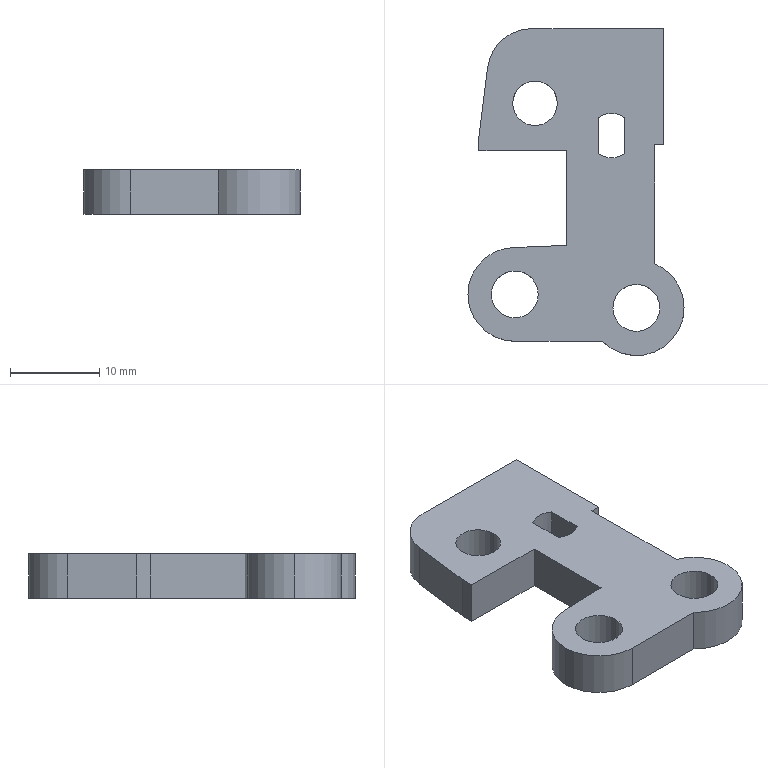Part | SolidWorks | features ICE 27, Join 2 | 1 solid | 27 faces | box 24.195 x 36.595 x 5 mm | volume 2687 mm3 | plane 14 | cylinder 13 | commonest cylinder face diameters 5 x4 5.25 x4 10.5 x2 10.691 x2 10 x1
STEP:
#1=CARTESIAN_POINT('',(-21.938,-6.808,-5.));
#2=VERTEX_POINT('',#1);
#3=CARTESIAN_POINT('',(-12.784,-3.058,-5.));
#4=VERTEX_POINT('',#3);
#5=CARTESIAN_POINT('',(-18.129,-3.058,-5.));
#6=DIRECTION('',(0.,0.,1.));
#7=DIRECTION('',(-1.,0.,0.));
#8=AXIS2_PLACEMENT_3D('',#5,#6,#7);
#9=CIRCLE('',#8,5.345);
#10=EDGE_CURVE('',#2,#4,#9,.T.);
#11=ORIENTED_EDGE('',*,*,#10,.T.);
#12=CARTESIAN_POINT('',(-12.784,-3.058,0.));
#13=VERTEX_POINT('',#12);
#14=CARTESIAN_POINT('',(-12.784,-3.058,-20.119));
#15=DIRECTION('',(0.,0.,1.));
#16=VECTOR('',#15,1000.);
#17=LINE('',#14,#16);
#18=EDGE_CURVE('',#4,#13,#17,.T.);
#19=ORIENTED_EDGE('',*,*,#18,.T.);
#20=CARTESIAN_POINT('',(-21.938,-6.808,0.));
#21=VERTEX_POINT('',#20);
#22=CARTESIAN_POINT('',(-18.129,-3.058,0.));
#23=DIRECTION('',(0.,0.,1.));
#24=DIRECTION('',(1.,0.,0.));
#25=AXIS2_PLACEMENT_3D('',#22,#23,#24);
#26=CIRCLE('',#25,5.345);
#27=EDGE_CURVE('',#21,#13,#26,.T.);
#28=ORIENTED_EDGE('',*,*,#27,.F.);
#29=CARTESIAN_POINT('',(-21.938,-6.808,-20.119));
#30=DIRECTION('',(0.,0.,1.));
#31=VECTOR('',#30,1000.);
#32=LINE('',#29,#31);
#33=EDGE_CURVE('',#2,#21,#32,.T.);
#34=ORIENTED_EDGE('',*,*,#33,.F.);
#35=EDGE_LOOP('',(#11,#19,#28,#34));
#36=FACE_OUTER_BOUND('',#35,.T.);
#37=CARTESIAN_POINT('',(-18.129,-3.058,-20.119));
#38=DIRECTION('',(0.,0.,1.));
#39=DIRECTION('',(1.,0.,0.));
#40=AXIS2_PLACEMENT_3D('',#37,#38,#39);
#41=CYLINDRICAL_SURFACE('',#40,5.345);
#42=ADVANCED_FACE('',(#36),#41,.T.);
#43=CARTESIAN_POINT('',(-36.979,-1.558,0.));
#44=VERTEX_POINT('',#43);
#45=CARTESIAN_POINT('',(-31.729,-6.808,0.));
#46=VERTEX_POINT('',#45);
#47=CARTESIAN_POINT('',(-31.729,-1.558,0.));
#48=DIRECTION('',(0.,0.,1.));
#49=DIRECTION('',(-1.,0.,0.));
#50=AXIS2_PLACEMENT_3D('',#47,#48,#49);
#51=CIRCLE('',#50,5.25);
#52=EDGE_CURVE('',#44,#46,#51,.T.);
#53=ORIENTED_EDGE('',*,*,#52,.F.);
#54=CARTESIAN_POINT('',(-36.979,-1.558,-5.));
#55=VERTEX_POINT('',#54);
#56=CARTESIAN_POINT('',(-36.979,-1.558,5.));
#57=DIRECTION('',(0.,0.,-1.));
#58=VECTOR('',#57,1000.);
#59=LINE('',#56,#58);
#60=EDGE_CURVE('',#44,#55,#59,.T.);
#61=ORIENTED_EDGE('',*,*,#60,.T.);
#62=CARTESIAN_POINT('',(-31.729,-6.808,-5.));
#63=VERTEX_POINT('',#62);
#64=CARTESIAN_POINT('',(-31.729,-1.558,-5.));
#65=DIRECTION('',(0.,0.,1.));
#66=DIRECTION('',(-1.,0.,0.));
#67=AXIS2_PLACEMENT_3D('',#64,#65,#66);
#68=CIRCLE('',#67,5.25);
#69=EDGE_CURVE('',#55,#63,#68,.T.);
#70=ORIENTED_EDGE('',*,*,#69,.T.);
#71=CARTESIAN_POINT('',(-31.729,-6.808,0.));
#72=DIRECTION('',(0.,0.,-1.));
#73=VECTOR('',#72,1000.);
#74=LINE('',#71,#73);
#75=EDGE_CURVE('',#46,#63,#74,.T.);
#76=ORIENTED_EDGE('',*,*,#75,.F.);
#77=EDGE_LOOP('',(#53,#61,#70,#76));
#78=FACE_OUTER_BOUND('',#77,.T.);
#79=CARTESIAN_POINT('',(-31.729,-1.558,5.));
#80=DIRECTION('',(0.,0.,-1.));
#81=DIRECTION('',(-1.,0.,0.));
#82=AXIS2_PLACEMENT_3D('',#79,#80,#81);
#83=CYLINDRICAL_SURFACE('',#82,5.25);
#84=ADVANCED_FACE('',(#78),#83,.T.);
#85=CARTESIAN_POINT('',(-20.754,-3.058,-5.));
#86=VERTEX_POINT('',#85);
#87=CARTESIAN_POINT('',(-15.504,-3.058,-5.));
#88=VERTEX_POINT('',#87);
#89=CARTESIAN_POINT('',(-18.129,-3.058,-5.));
#90=DIRECTION('',(0.,0.,1.));
#91=DIRECTION('',(1.,0.,0.));
#92=AXIS2_PLACEMENT_3D('',#89,#90,#91);
#93=CIRCLE('',#92,2.625);
#94=EDGE_CURVE('',#86,#88,#93,.T.);
#95=ORIENTED_EDGE('',*,*,#94,.F.);
#96=CARTESIAN_POINT('',(-20.754,-3.058,0.));
#97=VERTEX_POINT('',#96);
#98=CARTESIAN_POINT('',(-20.754,-3.058,-5.));
#99=DIRECTION('',(0.,0.,1.));
#100=VECTOR('',#99,1000.);
#101=LINE('',#98,#100);
#102=EDGE_CURVE('',#86,#97,#101,.T.);
#103=ORIENTED_EDGE('',*,*,#102,.T.);
#104=CARTESIAN_POINT('',(-15.504,-3.058,0.));
#105=VERTEX_POINT('',#104);
#106=CARTESIAN_POINT('',(-18.129,-3.058,0.));
#107=DIRECTION('',(0.,0.,1.));
#108=DIRECTION('',(1.,0.,0.));
#109=AXIS2_PLACEMENT_3D('',#106,#107,#108);
#110=CIRCLE('',#109,2.625);
#111=EDGE_CURVE('',#97,#105,#110,.T.);
#112=ORIENTED_EDGE('',*,*,#111,.T.);
#113=CARTESIAN_POINT('',(-15.504,-3.058,-5.));
#114=DIRECTION('',(0.,0.,1.));
#115=VECTOR('',#114,1000.);
#116=LINE('',#113,#115);
#117=EDGE_CURVE('',#88,#105,#116,.T.);
#118=ORIENTED_EDGE('',*,*,#117,.F.);
#119=EDGE_LOOP('',(#95,#103,#112,#118));
#120=FACE_OUTER_BOUND('',#119,.T.);
#121=CARTESIAN_POINT('',(-18.129,-3.058,-5.));
#122=DIRECTION('',(0.,0.,1.));
#123=DIRECTION('',(1.,0.,0.));
#124=AXIS2_PLACEMENT_3D('',#121,#122,#123);
#125=CYLINDRICAL_SURFACE('',#124,2.625);
#126=ADVANCED_FACE('',(#120),#125,.F.);
#127=CARTESIAN_POINT('',(-29.104,-1.558,-5.));
#128=VERTEX_POINT('',#127);
#129=CARTESIAN_POINT('',(-34.354,-1.558,-5.));
#130=VERTEX_POINT('',#129);
#131=CARTESIAN_POINT('',(-31.729,-1.558,-5.));
#132=DIRECTION('',(0.,0.,-1.));
#133=DIRECTION('',(-1.,0.,0.));
#134=AXIS2_PLACEMENT_3D('',#131,#132,#133);
#135=CIRCLE('',#134,2.625);
#136=EDGE_CURVE('',#128,#130,#135,.T.);
#137=ORIENTED_EDGE('',*,*,#136,.T.);
#138=CARTESIAN_POINT('',(-34.354,-1.558,0.));
#139=VERTEX_POINT('',#138);
#140=CARTESIAN_POINT('',(-34.354,-1.558,-19.));
#141=DIRECTION('',(0.,0.,1.));
#142=VECTOR('',#141,1000.);
#143=LINE('',#140,#142);
#144=EDGE_CURVE('',#130,#139,#143,.T.);
#145=ORIENTED_EDGE('',*,*,#144,.T.);
#146=CARTESIAN_POINT('',(-29.104,-1.558,0.));
#147=VERTEX_POINT('',#146);
#148=CARTESIAN_POINT('',(-31.729,-1.558,0.));
#149=DIRECTION('',(0.,0.,-1.));
#150=DIRECTION('',(-1.,0.,0.));
#151=AXIS2_PLACEMENT_3D('',#148,#149,#150);
#152=CIRCLE('',#151,2.625);
#153=EDGE_CURVE('',#147,#139,#152,.T.);
#154=ORIENTED_EDGE('',*,*,#153,.F.);
#155=CARTESIAN_POINT('',(-29.104,-1.558,-19.));
#156=DIRECTION('',(0.,0.,1.));
#157=VECTOR('',#156,1000.);
#158=LINE('',#155,#157);
#159=EDGE_CURVE('',#128,#147,#158,.T.);
#160=ORIENTED_EDGE('',*,*,#159,.F.);
#161=EDGE_LOOP('',(#137,#145,#154,#160));
#162=FACE_OUTER_BOUND('',#161,.T.);
#163=CARTESIAN_POINT('',(-31.729,-1.558,-19.));
#164=DIRECTION('',(0.,0.,1.));
#165=DIRECTION('',(1.,0.,0.));
#166=AXIS2_PLACEMENT_3D('',#163,#164,#165);
#167=CYLINDRICAL_SURFACE('',#166,2.625);
#168=ADVANCED_FACE('',(#162),#167,.F.);
#169=CARTESIAN_POINT('',(-31.965,19.823,-5.));
#170=VERTEX_POINT('',#169);
#171=CARTESIAN_POINT('',(-26.965,19.823,-5.));
#172=VERTEX_POINT('',#171);
#173=CARTESIAN_POINT('',(-29.465,19.823,-5.));
#174=DIRECTION('',(0.,0.,1.));
#175=DIRECTION('',(1.,0.,0.));
#176=AXIS2_PLACEMENT_3D('',#173,#174,#175);
#177=CIRCLE('',#176,2.5);
#178=EDGE_CURVE('',#170,#172,#177,.T.);
#179=ORIENTED_EDGE('',*,*,#178,.F.);
#180=CARTESIAN_POINT('',(-31.965,19.823,0.));
#181=VERTEX_POINT('',#180);
#182=CARTESIAN_POINT('',(-31.965,19.823,-10.));
#183=DIRECTION('',(0.,0.,1.));
#184=VECTOR('',#183,1000.);
#185=LINE('',#182,#184);
#186=EDGE_CURVE('',#170,#181,#185,.T.);
#187=ORIENTED_EDGE('',*,*,#186,.T.);
#188=CARTESIAN_POINT('',(-26.965,19.823,0.));
#189=VERTEX_POINT('',#188);
#190=CARTESIAN_POINT('',(-29.465,19.823,0.));
#191=DIRECTION('',(0.,0.,1.));
#192=DIRECTION('',(1.,0.,0.));
#193=AXIS2_PLACEMENT_3D('',#190,#191,#192);
#194=CIRCLE('',#193,2.5);
#195=EDGE_CURVE('',#181,#189,#194,.T.);
#196=ORIENTED_EDGE('',*,*,#195,.T.);
#197=CARTESIAN_POINT('',(-26.965,19.823,-10.));
#198=DIRECTION('',(0.,0.,1.));
#199=VECTOR('',#198,1000.);
#200=LINE('',#197,#199);
#201=EDGE_CURVE('',#172,#189,#200,.T.);
#202=ORIENTED_EDGE('',*,*,#201,.F.);
#203=EDGE_LOOP('',(#179,#187,#196,#202));
#204=FACE_OUTER_BOUND('',#203,.T.);
#205=CARTESIAN_POINT('',(-29.465,19.823,-10.));
#206=DIRECTION('',(0.,0.,1.));
#207=DIRECTION('',(1.,0.,0.));
#208=AXIS2_PLACEMENT_3D('',#205,#206,#207);
#209=CYLINDRICAL_SURFACE('',#208,2.5);
#210=ADVANCED_FACE('',(#204),#209,.F.);
#211=CARTESIAN_POINT('',(-15.057,28.192,0.));
#212=VERTEX_POINT('',#211);
#213=CARTESIAN_POINT('',(-15.057,28.192,-5.));
#214=VERTEX_POINT('',#213);
#215=CARTESIAN_POINT('',(-15.057,28.192,5.));
#216=DIRECTION('',(0.,0.,-1.));
#217=VECTOR('',#216,1000.);
#218=LINE('',#215,#217);
#219=EDGE_CURVE('',#212,#214,#218,.T.);
#220=ORIENTED_EDGE('',*,*,#219,.T.);
#221=CARTESIAN_POINT('',(-29.822,28.192,-5.));
#222=VERTEX_POINT('',#221);
#223=CARTESIAN_POINT('',(-16.089,28.192,-5.));
#224=DIRECTION('',(1.,0.,0.));
#225=VECTOR('',#224,1000.);
#226=LINE('',#223,#225);
#227=EDGE_CURVE('',#222,#214,#226,.T.);
#228=ORIENTED_EDGE('',*,*,#227,.F.);
#229=CARTESIAN_POINT('',(-29.822,28.192,0.));
#230=VERTEX_POINT('',#229);
#231=CARTESIAN_POINT('',(-29.822,28.192,0.));
#232=DIRECTION('',(0.,0.,1.));
#233=VECTOR('',#232,1000.);
#234=LINE('',#231,#233);
#235=EDGE_CURVE('',#222,#230,#234,.T.);
#236=ORIENTED_EDGE('',*,*,#235,.T.);
#237=CARTESIAN_POINT('',(-16.089,28.192,0.));
#238=DIRECTION('',(1.,0.,0.));
#239=VECTOR('',#238,1000.);
#240=LINE('',#237,#239);
#241=EDGE_CURVE('',#230,#212,#240,.T.);
#242=ORIENTED_EDGE('',*,*,#241,.T.);
#243=EDGE_LOOP('',(#220,#228,#236,#242));
#244=FACE_OUTER_BOUND('',#243,.T.);
#245=CARTESIAN_POINT('',(-16.089,28.192,-5.));
#246=DIRECTION('',(0.,-1.,0.));
#247=DIRECTION('',(0.,0.,-1.));
#248=AXIS2_PLACEMENT_3D('',#245,#246,#247);
#249=PLANE('',#248);
#250=ADVANCED_FACE('',(#244),#249,.F.);
#251=CARTESIAN_POINT('',(-15.057,15.192,0.));
#252=VERTEX_POINT('',#251);
#253=CARTESIAN_POINT('',(-15.057,15.192,-5.));
#254=VERTEX_POINT('',#253);
#255=CARTESIAN_POINT('',(-15.057,15.192,5.));
#256=DIRECTION('',(0.,0.,-1.));
#257=VECTOR('',#256,1000.);
#258=LINE('',#255,#257);
#259=EDGE_CURVE('',#252,#254,#258,.T.);
#260=ORIENTED_EDGE('',*,*,#259,.F.);
#261=CARTESIAN_POINT('',(-16.089,15.192,0.));
#262=VERTEX_POINT('',#261);
#263=CARTESIAN_POINT('',(-16.089,15.192,0.));
#264=DIRECTION('',(1.,0.,0.));
#265=VECTOR('',#264,1000.);
#266=LINE('',#263,#265);
#267=EDGE_CURVE('',#262,#252,#266,.T.);
#268=ORIENTED_EDGE('',*,*,#267,.F.);
#269=CARTESIAN_POINT('',(-16.089,15.192,-5.));
#270=VERTEX_POINT('',#269);
#271=CARTESIAN_POINT('',(-16.089,15.192,-5.));
#272=DIRECTION('',(0.,0.,1.));
#273=VECTOR('',#272,1000.);
#274=LINE('',#271,#273);
#275=EDGE_CURVE('',#270,#262,#274,.T.);
#276=ORIENTED_EDGE('',*,*,#275,.F.);
#277=CARTESIAN_POINT('',(-16.089,15.192,-5.));
#278=DIRECTION('',(1.,0.,0.));
#279=VECTOR('',#278,1000.);
#280=LINE('',#277,#279);
#281=EDGE_CURVE('',#270,#254,#280,.T.);
#282=ORIENTED_EDGE('',*,*,#281,.T.);
#283=EDGE_LOOP('',(#260,#268,#276,#282));
#284=FACE_OUTER_BOUND('',#283,.T.);
#285=CARTESIAN_POINT('',(-16.089,15.192,-5.));
#286=DIRECTION('',(0.,1.,0.));
#287=DIRECTION('',(0.,0.,1.));
#288=AXIS2_PLACEMENT_3D('',#285,#286,#287);
#289=PLANE('',#288);
#290=ADVANCED_FACE('',(#284),#289,.F.);
#291=CARTESIAN_POINT('',(-18.129,-3.058,-5.));
#292=DIRECTION('',(0.,0.,1.));
#293=DIRECTION('',(1.,0.,0.));
#294=AXIS2_PLACEMENT_3D('',#291,#292,#293);
#295=CIRCLE('',#294,2.625);
#296=EDGE_CURVE('',#88,#86,#295,.T.);
#297=ORIENTED_EDGE('',*,*,#296,.T.);
#298=ORIENTED_EDGE('',*,*,#94,.T.);
#299=EDGE_LOOP('',(#297,#298));
#300=FACE_BOUND('',#299,.T.);
#301=CARTESIAN_POINT('',(-29.465,19.823,-5.));
#302=DIRECTION('',(0.,0.,1.));
#303=DIRECTION('',(1.,0.,0.));
#304=AXIS2_PLACEMENT_3D('',#301,#302,#303);
#305=CIRCLE('',#304,2.5);
#306=EDGE_CURVE('',#172,#170,#305,.T.);
#307=ORIENTED_EDGE('',*,*,#306,.T.);
#308=ORIENTED_EDGE('',*,*,#178,.T.);
#309=EDGE_LOOP('',(#307,#308));
#310=FACE_BOUND('',#309,.T.);
#311=ORIENTED_EDGE('',*,*,#136,.F.);
#312=CARTESIAN_POINT('',(-31.729,-1.558,-5.));
#313=DIRECTION('',(0.,0.,-1.));
#314=DIRECTION('',(-1.,0.,0.));
#315=AXIS2_PLACEMENT_3D('',#312,#313,#314);
#316=CIRCLE('',#315,2.625);
#317=EDGE_CURVE('',#130,#128,#316,.T.);
#318=ORIENTED_EDGE('',*,*,#317,.F.);
#319=EDGE_LOOP('',(#311,#318));
#320=FACE_BOUND('',#319,.T.);
#321=CARTESIAN_POINT('',(-19.41,18.219,-5.));
#322=VERTEX_POINT('',#321);
#323=CARTESIAN_POINT('',(-22.41,18.219,-5.));
#324=VERTEX_POINT('',#323);
#325=CARTESIAN_POINT('',(-20.91,16.219,-5.));
#326=DIRECTION('',(0.,0.,1.));
#327=DIRECTION('',(1.,0.,0.));
#328=AXIS2_PLACEMENT_3D('',#325,#326,#327);
#329=CIRCLE('',#328,2.5);
#330=EDGE_CURVE('',#322,#324,#329,.T.);
#331=ORIENTED_EDGE('',*,*,#330,.T.);
#332=CARTESIAN_POINT('',(-22.41,14.219,-5.));
#333=VERTEX_POINT('',#332);
#334=CARTESIAN_POINT('',(-22.41,18.219,-5.));
#335=DIRECTION('',(0.,-1.,0.));
#336=VECTOR('',#335,1000.);
#337=LINE('',#334,#336);
#338=EDGE_CURVE('',#324,#333,#337,.T.);
#339=ORIENTED_EDGE('',*,*,#338,.T.);
#340=CARTESIAN_POINT('',(-19.41,14.219,-5.));
#341=VERTEX_POINT('',#340);
#342=CARTESIAN_POINT('',(-20.91,16.219,-5.));
#343=DIRECTION('',(0.,0.,1.));
#344=DIRECTION('',(1.,0.,0.));
#345=AXIS2_PLACEMENT_3D('',#342,#343,#344);
#346=CIRCLE('',#345,2.5);
#347=EDGE_CURVE('',#333,#341,#346,.T.);
#348=ORIENTED_EDGE('',*,*,#347,.T.);
#349=CARTESIAN_POINT('',(-19.41,18.219,-5.));
#350=DIRECTION('',(0.,1.,0.));
#351=VECTOR('',#350,1000.);
#352=LINE('',#349,#351);
#353=EDGE_CURVE('',#341,#322,#352,.T.);
#354=ORIENTED_EDGE('',*,*,#353,.T.);
#355=EDGE_LOOP('',(#331,#339,#348,#354));
#356=FACE_BOUND('',#355,.T.);
#357=ORIENTED_EDGE('',*,*,#227,.T.);
#358=CARTESIAN_POINT('',(-15.057,0.,-5.));
#359=DIRECTION('',(0.,-1.,0.));
#360=VECTOR('',#359,1000.);
#361=LINE('',#358,#360);
#362=EDGE_CURVE('',#214,#254,#361,.T.);
#363=ORIENTED_EDGE('',*,*,#362,.T.);
#364=ORIENTED_EDGE('',*,*,#281,.F.);
#365=CARTESIAN_POINT('',(-16.089,1.883,-5.));
#366=VERTEX_POINT('',#365);
#367=CARTESIAN_POINT('',(-16.089,10.692,-5.));
#368=DIRECTION('',(0.,-1.,0.));
#369=VECTOR('',#368,1000.);
#370=LINE('',#367,#369);
#371=EDGE_CURVE('',#270,#366,#370,.T.);
#372=ORIENTED_EDGE('',*,*,#371,.T.);
#373=CARTESIAN_POINT('',(-18.129,-3.058,-5.));
#374=DIRECTION('',(0.,0.,1.));
#375=DIRECTION('',(-1.,0.,0.));
#376=AXIS2_PLACEMENT_3D('',#373,#374,#375);
#377=CIRCLE('',#376,5.345);
#378=EDGE_CURVE('',#4,#366,#377,.T.);
#379=ORIENTED_EDGE('',*,*,#378,.F.);
#380=ORIENTED_EDGE('',*,*,#10,.F.);
#381=CARTESIAN_POINT('',(-21.089,-6.808,-5.));
#382=DIRECTION('',(1.,0.,0.));
#383=VECTOR('',#382,1000.);
#384=LINE('',#381,#383);
#385=EDGE_CURVE('',#63,#2,#384,.T.);
#386=ORIENTED_EDGE('',*,*,#385,.F.);
#387=ORIENTED_EDGE('',*,*,#69,.F.);
#388=CARTESIAN_POINT('',(-31.729,3.692,-5.));
#389=VERTEX_POINT('',#388);
#390=CARTESIAN_POINT('',(-31.729,-1.558,-5.));
#391=DIRECTION('',(0.,0.,1.));
#392=DIRECTION('',(-1.,0.,0.));
#393=AXIS2_PLACEMENT_3D('',#390,#391,#392);
#394=CIRCLE('',#393,5.25);
#395=EDGE_CURVE('',#389,#55,#394,.T.);
#396=ORIENTED_EDGE('',*,*,#395,.F.);
#397=CARTESIAN_POINT('',(-25.914,3.931,-5.));
#398=VERTEX_POINT('',#397);
#399=CARTESIAN_POINT('',(-31.729,3.692,-5.));
#400=DIRECTION('',(-0.9992,-0.04106,0.));
#401=VECTOR('',#400,1000.);
#402=LINE('',#399,#401);
#403=EDGE_CURVE('',#398,#389,#402,.T.);
#404=ORIENTED_EDGE('',*,*,#403,.F.);
#405=CARTESIAN_POINT('',(-25.914,14.531,-5.));
#406=VERTEX_POINT('',#405);
#407=CARTESIAN_POINT('',(-25.914,16.121,-5.));
#408=DIRECTION('',(0.,1.,0.));
#409=VECTOR('',#408,1000.);
#410=LINE('',#407,#409);
#411=EDGE_CURVE('',#398,#406,#410,.T.);
#412=ORIENTED_EDGE('',*,*,#411,.T.);
#413=CARTESIAN_POINT('',(-35.744,14.531,-5.));
#414=VERTEX_POINT('',#413);
#415=CARTESIAN_POINT('',(-35.744,14.531,-5.));
#416=DIRECTION('',(1.,0.,0.));
#417=VECTOR('',#416,1000.);
#418=LINE('',#415,#417);
#419=EDGE_CURVE('',#414,#406,#418,.T.);
#420=ORIENTED_EDGE('',*,*,#419,.F.);
#421=CARTESIAN_POINT('',(-35.744,16.086,-5.));
#422=VERTEX_POINT('',#421);
#423=CARTESIAN_POINT('',(-35.744,16.086,-5.));
#424=DIRECTION('',(0.,-1.,0.));
#425=VECTOR('',#424,1000.);
#426=LINE('',#423,#425);
#427=EDGE_CURVE('',#422,#414,#426,.T.);
#428=ORIENTED_EDGE('',*,*,#427,.F.);
#429=CARTESIAN_POINT('',(-34.784,23.809,-5.));
#430=VERTEX_POINT('',#429);
#431=CARTESIAN_POINT('',(-36.181,12.568,-5.));
#432=DIRECTION('',(0.1233,0.9924,0.));
#433=VECTOR('',#432,1000.);
#434=LINE('',#431,#433);
#435=EDGE_CURVE('',#422,#430,#434,.T.);
#436=ORIENTED_EDGE('',*,*,#435,.T.);
#437=CARTESIAN_POINT('',(-29.822,23.192,-5.));
#438=DIRECTION('',(0.,0.,-1.));
#439=DIRECTION('',(1.,0.,0.));
#440=AXIS2_PLACEMENT_3D('',#437,#438,#439);
#441=CIRCLE('',#440,5.);
#442=EDGE_CURVE('',#430,#222,#441,.T.);
#443=ORIENTED_EDGE('',*,*,#442,.T.);
#444=EDGE_LOOP('',(#357,#363,#364,#372,#379,#380,#386,#387,#396,#404,#412,#420,#428,#436,#443));
#445=FACE_OUTER_BOUND('',#444,.T.);
#446=CARTESIAN_POINT('',(33.02,-2.82,-5.));
#447=DIRECTION('',(0.,0.,-1.));
#448=DIRECTION('',(-0.9704,-0.2415,0.));
#449=AXIS2_PLACEMENT_3D('',#446,#447,#448);
#450=PLANE('',#449);
#451=ADVANCED_FACE('',(#300,#310,#320,#356,#445),#450,.T.);
#452=CARTESIAN_POINT('',(-18.129,-3.058,0.));
#453=DIRECTION('',(0.,0.,1.));
#454=DIRECTION('',(1.,0.,0.));
#455=AXIS2_PLACEMENT_3D('',#452,#453,#454);
#456=CIRCLE('',#455,2.625);
#457=EDGE_CURVE('',#105,#97,#456,.T.);
#458=ORIENTED_EDGE('',*,*,#457,.F.);
#459=ORIENTED_EDGE('',*,*,#111,.F.);
#460=EDGE_LOOP('',(#458,#459));
#461=FACE_BOUND('',#460,.T.);
#462=ORIENTED_EDGE('',*,*,#153,.T.);
#463=CARTESIAN_POINT('',(-31.729,-1.558,0.));
#464=DIRECTION('',(0.,0.,-1.));
#465=DIRECTION('',(-1.,0.,0.));
#466=AXIS2_PLACEMENT_3D('',#463,#464,#465);
#467=CIRCLE('',#466,2.625);
#468=EDGE_CURVE('',#139,#147,#467,.T.);
#469=ORIENTED_EDGE('',*,*,#468,.T.);
#470=EDGE_LOOP('',(#462,#469));
#471=FACE_BOUND('',#470,.T.);
#472=CARTESIAN_POINT('',(-29.465,19.823,0.));
#473=DIRECTION('',(0.,0.,1.));
#474=DIRECTION('',(1.,0.,0.));
#475=AXIS2_PLACEMENT_3D('',#472,#473,#474);
#476=CIRCLE('',#475,2.5);
#477=EDGE_CURVE('',#189,#181,#476,.T.);
#478=ORIENTED_EDGE('',*,*,#477,.F.);
#479=ORIENTED_EDGE('',*,*,#195,.F.);
#480=EDGE_LOOP('',(#478,#479));
#481=FACE_BOUND('',#480,.T.);
#482=CARTESIAN_POINT('',(-22.41,18.219,0.));
#483=VERTEX_POINT('',#482);
#484=CARTESIAN_POINT('',(-22.41,14.219,0.));
#485=VERTEX_POINT('',#484);
#486=CARTESIAN_POINT('',(-22.41,18.219,0.));
#487=DIRECTION('',(0.,-1.,0.));
#488=VECTOR('',#487,1000.);
#489=LINE('',#486,#488);
#490=EDGE_CURVE('',#483,#485,#489,.T.);
#491=ORIENTED_EDGE('',*,*,#490,.F.);
#492=CARTESIAN_POINT('',(-19.41,18.219,0.));
#493=VERTEX_POINT('',#492);
#494=CARTESIAN_POINT('',(-20.91,16.219,0.));
#495=DIRECTION('',(0.,0.,1.));
#496=DIRECTION('',(1.,0.,0.));
#497=AXIS2_PLACEMENT_3D('',#494,#495,#496);
#498=CIRCLE('',#497,2.5);
#499=EDGE_CURVE('',#493,#483,#498,.T.);
#500=ORIENTED_EDGE('',*,*,#499,.F.);
#501=CARTESIAN_POINT('',(-19.41,14.219,0.));
#502=VERTEX_POINT('',#501);
#503=CARTESIAN_POINT('',(-19.41,18.219,0.));
#504=DIRECTION('',(0.,1.,0.));
#505=VECTOR('',#504,1000.);
#506=LINE('',#503,#505);
#507=EDGE_CURVE('',#502,#493,#506,.T.);
#508=ORIENTED_EDGE('',*,*,#507,.F.);
#509=CARTESIAN_POINT('',(-20.91,16.219,0.));
#510=DIRECTION('',(0.,0.,1.));
#511=DIRECTION('',(1.,0.,0.));
#512=AXIS2_PLACEMENT_3D('',#509,#510,#511);
#513=CIRCLE('',#512,2.5);
#514=EDGE_CURVE('',#485,#502,#513,.T.);
#515=ORIENTED_EDGE('',*,*,#514,.F.);
#516=EDGE_LOOP('',(#491,#500,#508,#515));
#517=FACE_BOUND('',#516,.T.);
#518=CARTESIAN_POINT('',(-15.057,-2.82,0.));
#519=DIRECTION('',(0.,-1.,0.));
#520=VECTOR('',#519,1000.);
#521=LINE('',#518,#520);
#522=EDGE_CURVE('',#212,#252,#521,.T.);
#523=ORIENTED_EDGE('',*,*,#522,.F.);
#524=ORIENTED_EDGE('',*,*,#241,.F.);
#525=CARTESIAN_POINT('',(-34.784,23.809,0.));
#526=VERTEX_POINT('',#525);
#527=CARTESIAN_POINT('',(-29.822,23.192,0.));
#528=DIRECTION('',(0.,0.,1.));
#529=DIRECTION('',(1.,0.,0.));
#530=AXIS2_PLACEMENT_3D('',#527,#528,#529);
#531=CIRCLE('',#530,5.);
#532=EDGE_CURVE('',#230,#526,#531,.T.);
#533=ORIENTED_EDGE('',*,*,#532,.T.);
#534=CARTESIAN_POINT('',(-35.744,16.086,0.));
#535=VERTEX_POINT('',#534);
#536=CARTESIAN_POINT('',(-36.181,12.568,0.));
#537=DIRECTION('',(0.1233,0.9924,0.));
#538=VECTOR('',#537,1000.);
#539=LINE('',#536,#538);
#540=EDGE_CURVE('',#535,#526,#539,.T.);
#541=ORIENTED_EDGE('',*,*,#540,.F.);
#542=CARTESIAN_POINT('',(-35.744,14.531,0.));
#543=VERTEX_POINT('',#542);
#544=CARTESIAN_POINT('',(-35.744,16.086,0.));
#545=DIRECTION('',(0.,-1.,0.));
#546=VECTOR('',#545,1000.);
#547=LINE('',#544,#546);
#548=EDGE_CURVE('',#535,#543,#547,.T.);
#549=ORIENTED_EDGE('',*,*,#548,.T.);
#550=CARTESIAN_POINT('',(-25.914,14.531,0.));
#551=VERTEX_POINT('',#550);
#552=CARTESIAN_POINT('',(-35.744,14.531,0.));
#553=DIRECTION('',(1.,0.,0.));
#554=VECTOR('',#553,1000.);
#555=LINE('',#552,#554);
#556=EDGE_CURVE('',#543,#551,#555,.T.);
#557=ORIENTED_EDGE('',*,*,#556,.T.);
#558=CARTESIAN_POINT('',(-25.914,3.931,0.));
#559=VERTEX_POINT('',#558);
#560=CARTESIAN_POINT('',(-25.914,16.121,0.));
#561=DIRECTION('',(0.,1.,0.));
#562=VECTOR('',#561,1000.);
#563=LINE('',#560,#562);
#564=EDGE_CURVE('',#559,#551,#563,.T.);
#565=ORIENTED_EDGE('',*,*,#564,.F.);
#566=CARTESIAN_POINT('',(-31.729,3.692,0.));
#567=VERTEX_POINT('',#566);
#568=CARTESIAN_POINT('',(32.644,6.337,0.));
#569=DIRECTION('',(-0.9992,-0.04106,0.));
#570=VECTOR('',#569,1000.);
#571=LINE('',#568,#570);
#572=EDGE_CURVE('',#559,#567,#571,.T.);
#573=ORIENTED_EDGE('',*,*,#572,.T.);
#574=CARTESIAN_POINT('',(-31.729,-1.558,0.));
#575=DIRECTION('',(0.,0.,1.));
#576=DIRECTION('',(-1.,0.,0.));
#577=AXIS2_PLACEMENT_3D('',#574,#575,#576);
#578=CIRCLE('',#577,5.25);
#579=EDGE_CURVE('',#567,#44,#578,.T.);
#580=ORIENTED_EDGE('',*,*,#579,.T.);
#581=ORIENTED_EDGE('',*,*,#52,.T.);
#582=CARTESIAN_POINT('',(-21.089,-6.808,0.));
#583=DIRECTION('',(1.,0.,0.));
#584=VECTOR('',#583,1000.);
#585=LINE('',#582,#584);
#586=EDGE_CURVE('',#46,#21,#585,.T.);
#587=ORIENTED_EDGE('',*,*,#586,.T.);
#588=ORIENTED_EDGE('',*,*,#27,.T.);
#589=CARTESIAN_POINT('',(-16.089,1.883,0.));
#590=VERTEX_POINT('',#589);
#591=CARTESIAN_POINT('',(-18.129,-3.058,0.));
#592=DIRECTION('',(0.,0.,1.));
#593=DIRECTION('',(1.,0.,0.));
#594=AXIS2_PLACEMENT_3D('',#591,#592,#593);
#595=CIRCLE('',#594,5.345);
#596=EDGE_CURVE('',#13,#590,#595,.T.);
#597=ORIENTED_EDGE('',*,*,#596,.T.);
#598=CARTESIAN_POINT('',(-16.089,10.692,0.));
#599=DIRECTION('',(0.,-1.,0.));
#600=VECTOR('',#599,1000.);
#601=LINE('',#598,#600);
#602=EDGE_CURVE('',#262,#590,#601,.T.);
#603=ORIENTED_EDGE('',*,*,#602,.F.);
#604=ORIENTED_EDGE('',*,*,#267,.T.);
#605=EDGE_LOOP('',(#523,#524,#533,#541,#549,#557,#565,#573,#580,#581,#587,#588,#597,#603,#604));
#606=FACE_OUTER_BOUND('',#605,.T.);
#607=CARTESIAN_POINT('',(33.02,-2.82,0.));
#608=DIRECTION('',(0.,0.,-1.));
#609=DIRECTION('',(-0.9704,-0.2415,0.));
#610=AXIS2_PLACEMENT_3D('',#607,#608,#609);
#611=PLANE('',#610);
#612=ADVANCED_FACE('',(#461,#471,#481,#517,#606),#611,.F.);
#613=ORIENTED_EDGE('',*,*,#602,.T.);
#614=CARTESIAN_POINT('',(-16.089,1.883,-5.));
#615=DIRECTION('',(0.,0.,-1.));
#616=VECTOR('',#615,1000.);
#617=LINE('',#614,#616);
#618=EDGE_CURVE('',#590,#366,#617,.T.);
#619=ORIENTED_EDGE('',*,*,#618,.T.);
#620=ORIENTED_EDGE('',*,*,#371,.F.);
#621=ORIENTED_EDGE('',*,*,#275,.T.);
#622=EDGE_LOOP('',(#613,#619,#620,#621));
#623=FACE_OUTER_BOUND('',#622,.T.);
#624=CARTESIAN_POINT('',(-16.089,10.692,-5.));
#625=DIRECTION('',(-1.,0.,0.));
#626=DIRECTION('',(0.,0.,1.));
#627=AXIS2_PLACEMENT_3D('',#624,#625,#626);
#628=PLANE('',#627);
#629=ADVANCED_FACE('',(#623),#628,.F.);
#630=CARTESIAN_POINT('',(-35.744,16.086,0.));
#631=DIRECTION('',(0.,0.,-1.));
#632=VECTOR('',#631,1000.);
#633=LINE('',#630,#632);
#634=EDGE_CURVE('',#535,#422,#633,.T.);
#635=ORIENTED_EDGE('',*,*,#634,.F.);
#636=ORIENTED_EDGE('',*,*,#540,.T.);
#637=CARTESIAN_POINT('',(-34.784,23.809,0.));
#638=DIRECTION('',(0.,0.,-1.));
#639=VECTOR('',#638,1000.);
#640=LINE('',#637,#639);
#641=EDGE_CURVE('',#526,#430,#640,.T.);
#642=ORIENTED_EDGE('',*,*,#641,.T.);
#643=ORIENTED_EDGE('',*,*,#435,.F.);
#644=EDGE_LOOP('',(#635,#636,#642,#643));
#645=FACE_OUTER_BOUND('',#644,.T.);
#646=CARTESIAN_POINT('',(-36.181,12.568,0.));
#647=DIRECTION('',(-0.9924,0.1233,0.));
#648=DIRECTION('',(-0.1233,-0.9924,0.));
#649=AXIS2_PLACEMENT_3D('',#646,#647,#648);
#650=PLANE('',#649);
#651=ADVANCED_FACE('',(#645),#650,.T.);
#652=ORIENTED_EDGE('',*,*,#641,.F.);
#653=ORIENTED_EDGE('',*,*,#532,.F.);
#654=ORIENTED_EDGE('',*,*,#235,.F.);
#655=ORIENTED_EDGE('',*,*,#442,.F.);
#656=EDGE_LOOP('',(#652,#653,#654,#655));
#657=FACE_OUTER_BOUND('',#656,.T.);
#658=CARTESIAN_POINT('',(-29.822,23.192,0.));
#659=DIRECTION('',(0.,0.,-1.));
#660=DIRECTION('',(-1.,0.,0.));
#661=AXIS2_PLACEMENT_3D('',#658,#659,#660);
#662=CYLINDRICAL_SURFACE('',#661,5.);
#663=ADVANCED_FACE('',(#657),#662,.T.);
#664=ORIENTED_EDGE('',*,*,#385,.T.);
#665=ORIENTED_EDGE('',*,*,#33,.T.);
#666=ORIENTED_EDGE('',*,*,#586,.F.);
#667=ORIENTED_EDGE('',*,*,#75,.T.);
#668=EDGE_LOOP('',(#664,#665,#666,#667));
#669=FACE_OUTER_BOUND('',#668,.T.);
#670=CARTESIAN_POINT('',(-21.089,-6.808,0.));
#671=DIRECTION('',(0.,1.,0.));
#672=DIRECTION('',(0.,0.,1.));
#673=AXIS2_PLACEMENT_3D('',#670,#671,#672);
#674=PLANE('',#673);
#675=ADVANCED_FACE('',(#669),#674,.F.);
#676=ORIENTED_EDGE('',*,*,#186,.F.);
#677=ORIENTED_EDGE('',*,*,#306,.F.);
#678=ORIENTED_EDGE('',*,*,#201,.T.);
#679=ORIENTED_EDGE('',*,*,#477,.T.);
#680=EDGE_LOOP('',(#676,#677,#678,#679));
#681=FACE_OUTER_BOUND('',#680,.T.);
#682=CARTESIAN_POINT('',(-29.465,19.823,-10.));
#683=DIRECTION('',(0.,0.,1.));
#684=DIRECTION('',(1.,0.,0.));
#685=AXIS2_PLACEMENT_3D('',#682,#683,#684);
#686=CYLINDRICAL_SURFACE('',#685,2.5);
#687=ADVANCED_FACE('',(#681),#686,.F.);
#688=ORIENTED_EDGE('',*,*,#144,.F.);
#689=ORIENTED_EDGE('',*,*,#317,.T.);
#690=ORIENTED_EDGE('',*,*,#159,.T.);
#691=ORIENTED_EDGE('',*,*,#468,.F.);
#692=EDGE_LOOP('',(#688,#689,#690,#691));
#693=FACE_OUTER_BOUND('',#692,.T.);
#694=CARTESIAN_POINT('',(-31.729,-1.558,-19.));
#695=DIRECTION('',(0.,0.,1.));
#696=DIRECTION('',(1.,0.,0.));
#697=AXIS2_PLACEMENT_3D('',#694,#695,#696);
#698=CYLINDRICAL_SURFACE('',#697,2.625);
#699=ADVANCED_FACE('',(#693),#698,.F.);
#700=ORIENTED_EDGE('',*,*,#102,.F.);
#701=ORIENTED_EDGE('',*,*,#296,.F.);
#702=ORIENTED_EDGE('',*,*,#117,.T.);
#703=ORIENTED_EDGE('',*,*,#457,.T.);
#704=EDGE_LOOP('',(#700,#701,#702,#703));
#705=FACE_OUTER_BOUND('',#704,.T.);
#706=CARTESIAN_POINT('',(-18.129,-3.058,-5.));
#707=DIRECTION('',(0.,0.,1.));
#708=DIRECTION('',(1.,0.,0.));
#709=AXIS2_PLACEMENT_3D('',#706,#707,#708);
#710=CYLINDRICAL_SURFACE('',#709,2.625);
#711=ADVANCED_FACE('',(#705),#710,.F.);
#712=ORIENTED_EDGE('',*,*,#572,.F.);
#713=CARTESIAN_POINT('',(-25.914,3.931,0.));
#714=DIRECTION('',(0.,0.,-1.));
#715=VECTOR('',#714,1000.);
#716=LINE('',#713,#715);
#717=EDGE_CURVE('',#559,#398,#716,.T.);
#718=ORIENTED_EDGE('',*,*,#717,.T.);
#719=ORIENTED_EDGE('',*,*,#403,.T.);
#720=CARTESIAN_POINT('',(-31.729,3.692,5.));
#721=DIRECTION('',(0.,0.,-1.));
#722=VECTOR('',#721,1000.);
#723=LINE('',#720,#722);
#724=EDGE_CURVE('',#567,#389,#723,.T.);
#725=ORIENTED_EDGE('',*,*,#724,.F.);
#726=EDGE_LOOP('',(#712,#718,#719,#725));
#727=FACE_OUTER_BOUND('',#726,.T.);
#728=CARTESIAN_POINT('',(-31.729,3.692,5.));
#729=DIRECTION('',(0.04106,-0.9992,0.));
#730=DIRECTION('',(0.9992,0.04106,0.));
#731=AXIS2_PLACEMENT_3D('',#728,#729,#730);
#732=PLANE('',#731);
#733=ADVANCED_FACE('',(#727),#732,.F.);
#734=ORIENTED_EDGE('',*,*,#60,.F.);
#735=ORIENTED_EDGE('',*,*,#579,.F.);
#736=ORIENTED_EDGE('',*,*,#724,.T.);
#737=ORIENTED_EDGE('',*,*,#395,.T.);
#738=EDGE_LOOP('',(#734,#735,#736,#737));
#739=FACE_OUTER_BOUND('',#738,.T.);
#740=CARTESIAN_POINT('',(-31.729,-1.558,5.));
#741=DIRECTION('',(0.,0.,-1.));
#742=DIRECTION('',(-1.,0.,0.));
#743=AXIS2_PLACEMENT_3D('',#740,#741,#742);
#744=CYLINDRICAL_SURFACE('',#743,5.25);
#745=ADVANCED_FACE('',(#739),#744,.T.);
#746=CARTESIAN_POINT('',(-25.914,14.531,-14.957));
#747=DIRECTION('',(0.,0.,1.));
#748=VECTOR('',#747,1000.);
#749=LINE('',#746,#748);
#750=EDGE_CURVE('',#406,#551,#749,.T.);
#751=ORIENTED_EDGE('',*,*,#750,.F.);
#752=ORIENTED_EDGE('',*,*,#411,.F.);
#753=ORIENTED_EDGE('',*,*,#717,.F.);
#754=ORIENTED_EDGE('',*,*,#564,.T.);
#755=EDGE_LOOP('',(#751,#752,#753,#754));
#756=FACE_OUTER_BOUND('',#755,.T.);
#757=CARTESIAN_POINT('',(-25.914,16.121,0.));
#758=DIRECTION('',(-1.,0.,0.));
#759=DIRECTION('',(0.,0.,1.));
#760=AXIS2_PLACEMENT_3D('',#757,#758,#759);
#761=PLANE('',#760);
#762=ADVANCED_FACE('',(#756),#761,.T.);
#763=ORIENTED_EDGE('',*,*,#634,.T.);
#764=ORIENTED_EDGE('',*,*,#427,.T.);
#765=CARTESIAN_POINT('',(-35.744,14.531,-14.957));
#766=DIRECTION('',(0.,0.,1.));
#767=VECTOR('',#766,1000.);
#768=LINE('',#765,#767);
#769=EDGE_CURVE('',#414,#543,#768,.T.);
#770=ORIENTED_EDGE('',*,*,#769,.T.);
#771=ORIENTED_EDGE('',*,*,#548,.F.);
#772=EDGE_LOOP('',(#763,#764,#770,#771));
#773=FACE_OUTER_BOUND('',#772,.T.);
#774=CARTESIAN_POINT('',(-35.744,16.086,-14.957));
#775=DIRECTION('',(-1.,0.,0.));
#776=DIRECTION('',(0.,0.,1.));
#777=AXIS2_PLACEMENT_3D('',#774,#775,#776);
#778=PLANE('',#777);
#779=ADVANCED_FACE('',(#773),#778,.T.);
#780=ORIENTED_EDGE('',*,*,#769,.F.);
#781=ORIENTED_EDGE('',*,*,#419,.T.);
#782=ORIENTED_EDGE('',*,*,#750,.T.);
#783=ORIENTED_EDGE('',*,*,#556,.F.);
#784=EDGE_LOOP('',(#780,#781,#782,#783));
#785=FACE_OUTER_BOUND('',#784,.T.);
#786=CARTESIAN_POINT('',(-35.744,14.531,-14.957));
#787=DIRECTION('',(0.,-1.,0.));
#788=DIRECTION('',(0.,0.,-1.));
#789=AXIS2_PLACEMENT_3D('',#786,#787,#788);
#790=PLANE('',#789);
#791=ADVANCED_FACE('',(#785),#790,.T.);
#792=ORIENTED_EDGE('',*,*,#499,.T.);
#793=CARTESIAN_POINT('',(-22.41,18.219,-5.));
#794=DIRECTION('',(0.,0.,1.));
#795=VECTOR('',#794,1000.);
#796=LINE('',#793,#795);
#797=EDGE_CURVE('',#324,#483,#796,.T.);
#798=ORIENTED_EDGE('',*,*,#797,.F.);
#799=ORIENTED_EDGE('',*,*,#330,.F.);
#800=CARTESIAN_POINT('',(-19.41,18.219,-5.));
#801=DIRECTION('',(0.,0.,1.));
#802=VECTOR('',#801,1000.);
#803=LINE('',#800,#802);
#804=EDGE_CURVE('',#322,#493,#803,.T.);
#805=ORIENTED_EDGE('',*,*,#804,.T.);
#806=EDGE_LOOP('',(#792,#798,#799,#805));
#807=FACE_OUTER_BOUND('',#806,.T.);
#808=CARTESIAN_POINT('',(-20.91,16.219,-5.));
#809=DIRECTION('',(0.,0.,1.));
#810=DIRECTION('',(1.,0.,0.));
#811=AXIS2_PLACEMENT_3D('',#808,#809,#810);
#812=CYLINDRICAL_SURFACE('',#811,2.5);
#813=ADVANCED_FACE('',(#807),#812,.F.);
#814=ORIENTED_EDGE('',*,*,#507,.T.);
#815=ORIENTED_EDGE('',*,*,#804,.F.);
#816=ORIENTED_EDGE('',*,*,#353,.F.);
#817=CARTESIAN_POINT('',(-19.41,14.219,-5.));
#818=DIRECTION('',(0.,0.,1.));
#819=VECTOR('',#818,1000.);
#820=LINE('',#817,#819);
#821=EDGE_CURVE('',#341,#502,#820,.T.);
#822=ORIENTED_EDGE('',*,*,#821,.T.);
#823=EDGE_LOOP('',(#814,#815,#816,#822));
#824=FACE_OUTER_BOUND('',#823,.T.);
#825=CARTESIAN_POINT('',(-19.41,18.219,-5.));
#826=DIRECTION('',(1.,0.,0.));
#827=DIRECTION('',(0.,0.,-1.));
#828=AXIS2_PLACEMENT_3D('',#825,#826,#827);
#829=PLANE('',#828);
#830=ADVANCED_FACE('',(#824),#829,.F.);
#831=ORIENTED_EDGE('',*,*,#514,.T.);
#832=ORIENTED_EDGE('',*,*,#821,.F.);
#833=ORIENTED_EDGE('',*,*,#347,.F.);
#834=CARTESIAN_POINT('',(-22.41,14.219,-5.));
#835=DIRECTION('',(0.,0.,1.));
#836=VECTOR('',#835,1000.);
#837=LINE('',#834,#836);
#838=EDGE_CURVE('',#333,#485,#837,.T.);
#839=ORIENTED_EDGE('',*,*,#838,.T.);
#840=EDGE_LOOP('',(#831,#832,#833,#839));
#841=FACE_OUTER_BOUND('',#840,.T.);
#842=CARTESIAN_POINT('',(-20.91,16.219,-5.));
#843=DIRECTION('',(0.,0.,1.));
#844=DIRECTION('',(1.,0.,0.));
#845=AXIS2_PLACEMENT_3D('',#842,#843,#844);
#846=CYLINDRICAL_SURFACE('',#845,2.5);
#847=ADVANCED_FACE('',(#841),#846,.F.);
#848=ORIENTED_EDGE('',*,*,#490,.T.);
#849=ORIENTED_EDGE('',*,*,#838,.F.);
#850=ORIENTED_EDGE('',*,*,#338,.F.);
#851=ORIENTED_EDGE('',*,*,#797,.T.);
#852=EDGE_LOOP('',(#848,#849,#850,#851));
#853=FACE_OUTER_BOUND('',#852,.T.);
#854=CARTESIAN_POINT('',(-22.41,18.219,-5.));
#855=DIRECTION('',(-1.,0.,0.));
#856=DIRECTION('',(0.,0.,1.));
#857=AXIS2_PLACEMENT_3D('',#854,#855,#856);
#858=PLANE('',#857);
#859=ADVANCED_FACE('',(#853),#858,.F.);
#860=ORIENTED_EDGE('',*,*,#18,.F.);
#861=ORIENTED_EDGE('',*,*,#378,.T.);
#862=ORIENTED_EDGE('',*,*,#618,.F.);
#863=ORIENTED_EDGE('',*,*,#596,.F.);
#864=EDGE_LOOP('',(#860,#861,#862,#863));
#865=FACE_OUTER_BOUND('',#864,.T.);
#866=CARTESIAN_POINT('',(-18.129,-3.058,-20.119));
#867=DIRECTION('',(0.,0.,1.));
#868=DIRECTION('',(1.,0.,0.));
#869=AXIS2_PLACEMENT_3D('',#866,#867,#868);
#870=CYLINDRICAL_SURFACE('',#869,5.345);
#871=ADVANCED_FACE('',(#865),#870,.T.);
#872=ORIENTED_EDGE('',*,*,#522,.T.);
#873=ORIENTED_EDGE('',*,*,#259,.T.);
#874=ORIENTED_EDGE('',*,*,#362,.F.);
#875=ORIENTED_EDGE('',*,*,#219,.F.);
#876=EDGE_LOOP('',(#872,#873,#874,#875));
#877=FACE_OUTER_BOUND('',#876,.T.);
#878=CARTESIAN_POINT('',(-15.057,0.,5.));
#879=DIRECTION('',(1.,0.,0.));
#880=DIRECTION('',(0.,0.,-1.));
#881=AXIS2_PLACEMENT_3D('',#878,#879,#880);
#882=PLANE('',#881);
#883=ADVANCED_FACE('',(#877),#882,.T.);
#884=CLOSED_SHELL('',(#42,#84,#126,#168,#210,#250,#290,#451,#612,#629,#651,#663,#675,#687,#699,#711,#733,#745,#762,#779,#791,#813,#830,#847,#859,#871,#883));
#885=MANIFOLD_SOLID_BREP('',#884);
#886=CARTESIAN_POINT('',(0.,0.,0.));
#887=DIRECTION('',(0.,0.,1.));
#888=DIRECTION('',(1.,0.,0.));
#889=AXIS2_PLACEMENT_3D('',#886,#887,#888);
#890=(LENGTH_UNIT()NAMED_UNIT(*)SI_UNIT(.MILLI.,.METRE.));
#891=UNCERTAINTY_MEASURE_WITH_UNIT(LENGTH_MEASURE(0.00001),#890,'','');
#892=(NAMED_UNIT(*)PLANE_ANGLE_UNIT()SI_UNIT($,.RADIAN.));
#893=(NAMED_UNIT(*)SI_UNIT($,.STERADIAN.)SOLID_ANGLE_UNIT());
#894=(GEOMETRIC_REPRESENTATION_CONTEXT(3)GLOBAL_UNCERTAINTY_ASSIGNED_CONTEXT((#891))GLOBAL_UNIT_ASSIGNED_CONTEXT((#890,#892,#893))REPRESENTATION_CONTEXT('',''));
#895=ADVANCED_BREP_SHAPE_REPRESENTATION('',(#885,#889),#894);